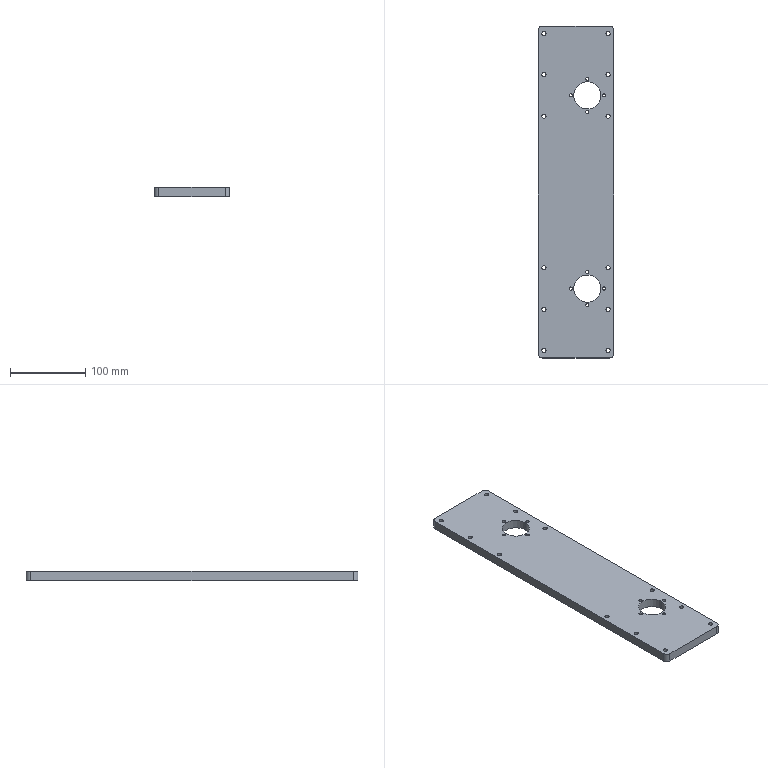Part | STEP file | QA-FC04 | 1 solid | 90 faces | box 100 x 440 x 12 mm | volume 495046 mm3 | cylinder 72 | plane 18 | commonest cylinder face diameters 5.5 x24 4.2 x16 10 x16 9.5 x8 12 x4 36 x4